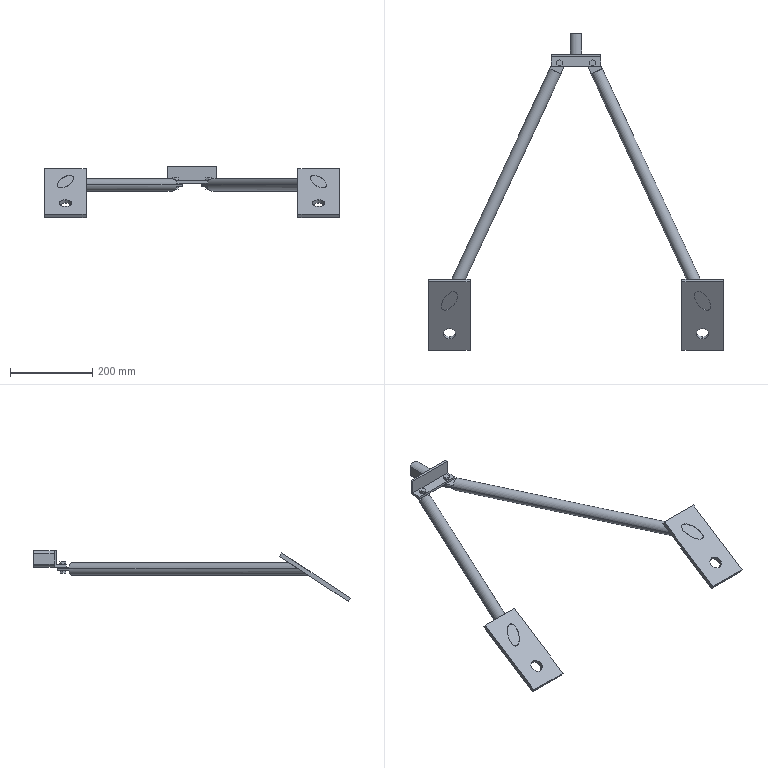Part | SolidWorks | features ICE 15, Cut 2, MoveFace 2, Sweep 2, BossThin 1, Scale 1 | 2 solids | 105 faces | box 715.381 x 770.357 x 124.108 mm | volume 1334452 mm3 | plane 74 | cylinder 20 | spline 11 | commonest cylinder face diameters 30 x8 7.5 x4 9 x4 12 x4